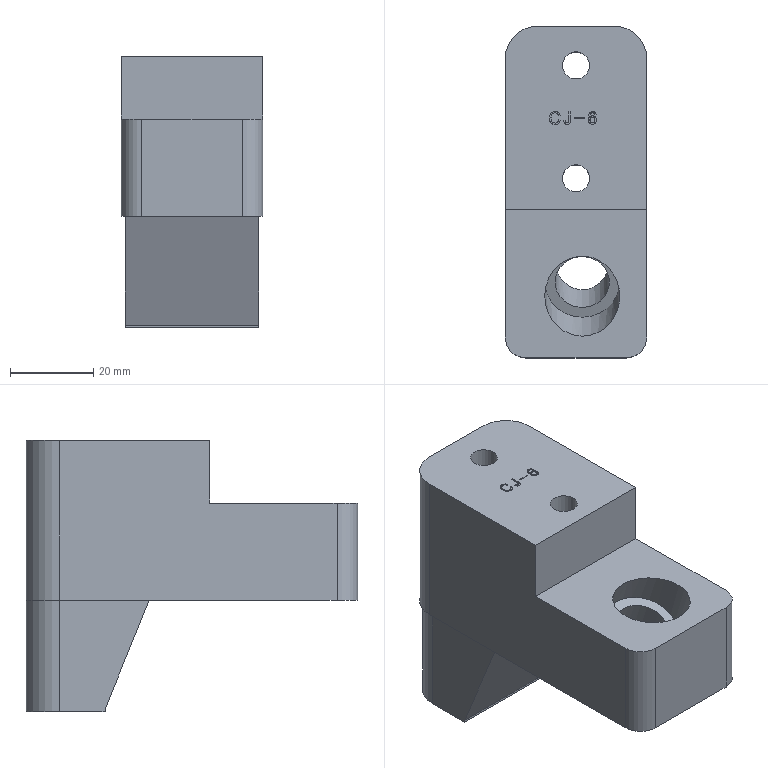Part | STEP file | solid 191 | 1 solid | 52 faces | box 34 x 79.555 x 65 mm | volume 95277 mm3 | plane 32 | cylinder 12 | other 8 | commonest cylinder face diameters 16 x4 6.5 x2 10 x2 11 x2 13 x1 18 x1